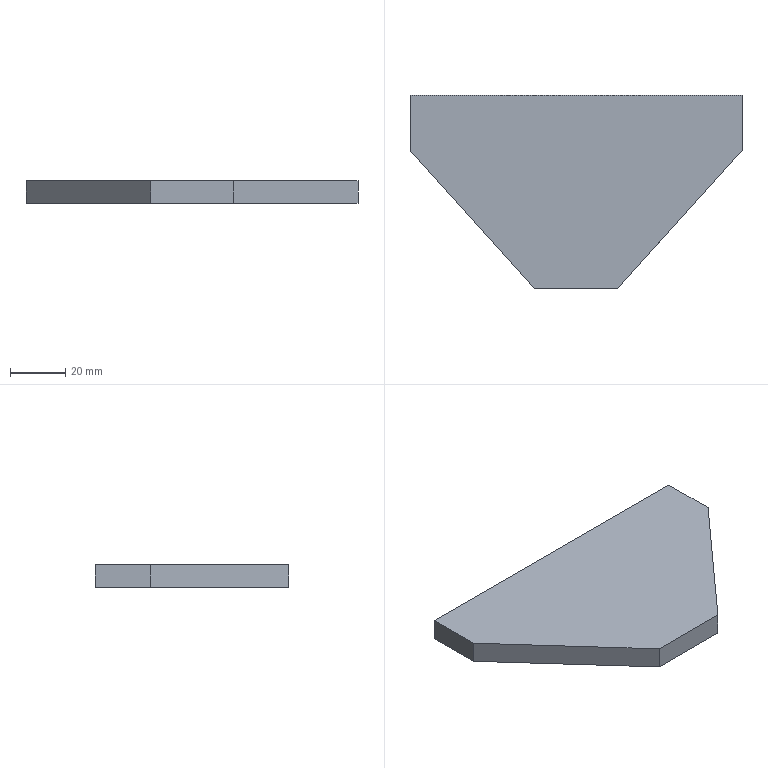Part | SolidWorks | features Extrusion 1, ICE 1 | 1 solid | 8 faces | box 120 x 70 x 8 mm | volume 49200 mm3 | plane 8
STEP:
#1=CARTESIAN_POINT('',(60.,15.,8.));
#2=VERTEX_POINT('',#1);
#3=CARTESIAN_POINT('',(60.,35.,8.));
#4=VERTEX_POINT('',#3);
#5=CARTESIAN_POINT('',(60.,35.,8.));
#6=DIRECTION('',(0.,1.,0.));
#7=VECTOR('',#6,1000.);
#8=LINE('',#5,#7);
#9=EDGE_CURVE('',#2,#4,#8,.T.);
#10=ORIENTED_EDGE('',*,*,#9,.F.);
#11=CARTESIAN_POINT('',(60.,15.,0.));
#12=VERTEX_POINT('',#11);
#13=CARTESIAN_POINT('',(60.,15.,0.));
#14=DIRECTION('',(0.,0.,1.));
#15=VECTOR('',#14,1000.);
#16=LINE('',#13,#15);
#17=EDGE_CURVE('',#12,#2,#16,.T.);
#18=ORIENTED_EDGE('',*,*,#17,.F.);
#19=CARTESIAN_POINT('',(60.,35.,0.));
#20=VERTEX_POINT('',#19);
#21=CARTESIAN_POINT('',(60.,35.,0.));
#22=DIRECTION('',(0.,1.,0.));
#23=VECTOR('',#22,1000.);
#24=LINE('',#21,#23);
#25=EDGE_CURVE('',#12,#20,#24,.T.);
#26=ORIENTED_EDGE('',*,*,#25,.T.);
#27=CARTESIAN_POINT('',(60.,35.,8.));
#28=DIRECTION('',(0.,0.,-1.));
#29=VECTOR('',#28,1000.);
#30=LINE('',#27,#29);
#31=EDGE_CURVE('',#4,#20,#30,.T.);
#32=ORIENTED_EDGE('',*,*,#31,.F.);
#33=EDGE_LOOP('',(#10,#18,#26,#32));
#34=FACE_OUTER_BOUND('',#33,.T.);
#35=CARTESIAN_POINT('',(60.,35.,8.));
#36=DIRECTION('',(-1.,0.,0.));
#37=DIRECTION('',(0.,-1.,0.));
#38=AXIS2_PLACEMENT_3D('',#35,#36,#37);
#39=PLANE('',#38);
#40=ADVANCED_FACE('',(#34),#39,.F.);
#41=CARTESIAN_POINT('',(-60.,35.,0.));
#42=VERTEX_POINT('',#41);
#43=CARTESIAN_POINT('',(-60.,35.,0.));
#44=DIRECTION('',(-1.,0.,0.));
#45=VECTOR('',#44,1000.);
#46=LINE('',#43,#45);
#47=EDGE_CURVE('',#20,#42,#46,.T.);
#48=ORIENTED_EDGE('',*,*,#47,.T.);
#49=CARTESIAN_POINT('',(-60.,35.,8.));
#50=VERTEX_POINT('',#49);
#51=CARTESIAN_POINT('',(-60.,35.,8.));
#52=DIRECTION('',(0.,0.,-1.));
#53=VECTOR('',#52,1000.);
#54=LINE('',#51,#53);
#55=EDGE_CURVE('',#50,#42,#54,.T.);
#56=ORIENTED_EDGE('',*,*,#55,.F.);
#57=CARTESIAN_POINT('',(-60.,35.,8.));
#58=DIRECTION('',(-1.,0.,0.));
#59=VECTOR('',#58,1000.);
#60=LINE('',#57,#59);
#61=EDGE_CURVE('',#4,#50,#60,.T.);
#62=ORIENTED_EDGE('',*,*,#61,.F.);
#63=ORIENTED_EDGE('',*,*,#31,.T.);
#64=EDGE_LOOP('',(#48,#56,#62,#63));
#65=FACE_OUTER_BOUND('',#64,.T.);
#66=CARTESIAN_POINT('',(-60.,35.,8.));
#67=DIRECTION('',(0.,-1.,0.));
#68=DIRECTION('',(0.,0.,-1.));
#69=AXIS2_PLACEMENT_3D('',#66,#67,#68);
#70=PLANE('',#69);
#71=ADVANCED_FACE('',(#65),#70,.F.);
#72=CARTESIAN_POINT('',(-60.,15.,0.));
#73=VERTEX_POINT('',#72);
#74=CARTESIAN_POINT('',(-60.,35.,0.));
#75=DIRECTION('',(0.,-1.,0.));
#76=VECTOR('',#75,1000.);
#77=LINE('',#74,#76);
#78=EDGE_CURVE('',#42,#73,#77,.T.);
#79=ORIENTED_EDGE('',*,*,#78,.T.);
#80=CARTESIAN_POINT('',(-60.,15.,8.));
#81=VERTEX_POINT('',#80);
#82=CARTESIAN_POINT('',(-60.,15.,0.));
#83=DIRECTION('',(0.,0.,1.));
#84=VECTOR('',#83,1000.);
#85=LINE('',#82,#84);
#86=EDGE_CURVE('',#73,#81,#85,.T.);
#87=ORIENTED_EDGE('',*,*,#86,.T.);
#88=CARTESIAN_POINT('',(-60.,35.,8.));
#89=DIRECTION('',(0.,-1.,0.));
#90=VECTOR('',#89,1000.);
#91=LINE('',#88,#90);
#92=EDGE_CURVE('',#50,#81,#91,.T.);
#93=ORIENTED_EDGE('',*,*,#92,.F.);
#94=ORIENTED_EDGE('',*,*,#55,.T.);
#95=EDGE_LOOP('',(#79,#87,#93,#94));
#96=FACE_OUTER_BOUND('',#95,.T.);
#97=CARTESIAN_POINT('',(-60.,35.,8.));
#98=DIRECTION('',(1.,0.,0.));
#99=DIRECTION('',(0.,1.,0.));
#100=AXIS2_PLACEMENT_3D('',#97,#98,#99);
#101=PLANE('',#100);
#102=ADVANCED_FACE('',(#96),#101,.F.);
#103=CARTESIAN_POINT('',(-15.,-35.,8.));
#104=VERTEX_POINT('',#103);
#105=CARTESIAN_POINT('',(15.,-35.,8.));
#106=VERTEX_POINT('',#105);
#107=CARTESIAN_POINT('',(-60.,-35.,8.));
#108=DIRECTION('',(1.,0.,0.));
#109=VECTOR('',#108,1000.);
#110=LINE('',#107,#109);
#111=EDGE_CURVE('',#104,#106,#110,.T.);
#112=ORIENTED_EDGE('',*,*,#111,.F.);
#113=CARTESIAN_POINT('',(-15.,-35.,0.));
#114=VERTEX_POINT('',#113);
#115=CARTESIAN_POINT('',(-15.,-35.,0.));
#116=DIRECTION('',(0.,0.,1.));
#117=VECTOR('',#116,1000.);
#118=LINE('',#115,#117);
#119=EDGE_CURVE('',#114,#104,#118,.T.);
#120=ORIENTED_EDGE('',*,*,#119,.F.);
#121=CARTESIAN_POINT('',(15.,-35.,0.));
#122=VERTEX_POINT('',#121);
#123=CARTESIAN_POINT('',(-60.,-35.,0.));
#124=DIRECTION('',(1.,0.,0.));
#125=VECTOR('',#124,1000.);
#126=LINE('',#123,#125);
#127=EDGE_CURVE('',#114,#122,#126,.T.);
#128=ORIENTED_EDGE('',*,*,#127,.T.);
#129=CARTESIAN_POINT('',(15.,-35.,0.));
#130=DIRECTION('',(0.,0.,1.));
#131=VECTOR('',#130,1000.);
#132=LINE('',#129,#131);
#133=EDGE_CURVE('',#122,#106,#132,.T.);
#134=ORIENTED_EDGE('',*,*,#133,.T.);
#135=EDGE_LOOP('',(#112,#120,#128,#134));
#136=FACE_OUTER_BOUND('',#135,.T.);
#137=CARTESIAN_POINT('',(-60.,-35.,8.));
#138=DIRECTION('',(0.,1.,0.));
#139=DIRECTION('',(0.,0.,1.));
#140=AXIS2_PLACEMENT_3D('',#137,#138,#139);
#141=PLANE('',#140);
#142=ADVANCED_FACE('',(#136),#141,.F.);
#143=CARTESIAN_POINT('',(-60.,15.,8.));
#144=DIRECTION('',(-0.669,0.7433,0.));
#145=VECTOR('',#144,1000.);
#146=LINE('',#143,#145);
#147=EDGE_CURVE('',#104,#81,#146,.T.);
#148=ORIENTED_EDGE('',*,*,#147,.F.);
#149=ORIENTED_EDGE('',*,*,#111,.T.);
#150=CARTESIAN_POINT('',(15.,-35.,8.));
#151=DIRECTION('',(-0.669,-0.7433,0.));
#152=VECTOR('',#151,1000.);
#153=LINE('',#150,#152);
#154=EDGE_CURVE('',#2,#106,#153,.T.);
#155=ORIENTED_EDGE('',*,*,#154,.F.);
#156=ORIENTED_EDGE('',*,*,#9,.T.);
#157=ORIENTED_EDGE('',*,*,#61,.T.);
#158=ORIENTED_EDGE('',*,*,#92,.T.);
#159=EDGE_LOOP('',(#148,#149,#155,#156,#157,#158));
#160=FACE_OUTER_BOUND('',#159,.T.);
#161=CARTESIAN_POINT('',(0.,0.,8.));
#162=DIRECTION('',(0.,0.,1.));
#163=DIRECTION('',(1.,0.,0.));
#164=AXIS2_PLACEMENT_3D('',#161,#162,#163);
#165=PLANE('',#164);
#166=ADVANCED_FACE('',(#160),#165,.T.);
#167=ORIENTED_EDGE('',*,*,#127,.F.);
#168=CARTESIAN_POINT('',(-60.,15.,0.));
#169=DIRECTION('',(-0.669,0.7433,0.));
#170=VECTOR('',#169,1000.);
#171=LINE('',#168,#170);
#172=EDGE_CURVE('',#114,#73,#171,.T.);
#173=ORIENTED_EDGE('',*,*,#172,.T.);
#174=ORIENTED_EDGE('',*,*,#78,.F.);
#175=ORIENTED_EDGE('',*,*,#47,.F.);
#176=ORIENTED_EDGE('',*,*,#25,.F.);
#177=CARTESIAN_POINT('',(15.,-35.,0.));
#178=DIRECTION('',(-0.669,-0.7433,0.));
#179=VECTOR('',#178,1000.);
#180=LINE('',#177,#179);
#181=EDGE_CURVE('',#12,#122,#180,.T.);
#182=ORIENTED_EDGE('',*,*,#181,.T.);
#183=EDGE_LOOP('',(#167,#173,#174,#175,#176,#182));
#184=FACE_OUTER_BOUND('',#183,.T.);
#185=CARTESIAN_POINT('',(0.,0.,0.));
#186=DIRECTION('',(0.,0.,1.));
#187=DIRECTION('',(1.,0.,0.));
#188=AXIS2_PLACEMENT_3D('',#185,#186,#187);
#189=PLANE('',#188);
#190=ADVANCED_FACE('',(#184),#189,.F.);
#191=ORIENTED_EDGE('',*,*,#154,.T.);
#192=ORIENTED_EDGE('',*,*,#133,.F.);
#193=ORIENTED_EDGE('',*,*,#181,.F.);
#194=ORIENTED_EDGE('',*,*,#17,.T.);
#195=EDGE_LOOP('',(#191,#192,#193,#194));
#196=FACE_OUTER_BOUND('',#195,.T.);
#197=CARTESIAN_POINT('',(15.,-35.,0.));
#198=DIRECTION('',(-0.7433,0.669,0.));
#199=DIRECTION('',(-0.669,-0.7433,0.));
#200=AXIS2_PLACEMENT_3D('',#197,#198,#199);
#201=PLANE('',#200);
#202=ADVANCED_FACE('',(#196),#201,.F.);
#203=ORIENTED_EDGE('',*,*,#147,.T.);
#204=ORIENTED_EDGE('',*,*,#86,.F.);
#205=ORIENTED_EDGE('',*,*,#172,.F.);
#206=ORIENTED_EDGE('',*,*,#119,.T.);
#207=EDGE_LOOP('',(#203,#204,#205,#206));
#208=FACE_OUTER_BOUND('',#207,.T.);
#209=CARTESIAN_POINT('',(-60.,15.,0.));
#210=DIRECTION('',(0.7433,0.669,0.));
#211=DIRECTION('',(-0.669,0.7433,0.));
#212=AXIS2_PLACEMENT_3D('',#209,#210,#211);
#213=PLANE('',#212);
#214=ADVANCED_FACE('',(#208),#213,.F.);
#215=CLOSED_SHELL('',(#40,#71,#102,#142,#166,#190,#202,#214));
#216=MANIFOLD_SOLID_BREP('',#215);
#217=CARTESIAN_POINT('',(0.,0.,0.));
#218=DIRECTION('',(0.,0.,1.));
#219=DIRECTION('',(1.,0.,0.));
#220=AXIS2_PLACEMENT_3D('',#217,#218,#219);
#221=(LENGTH_UNIT()NAMED_UNIT(*)SI_UNIT(.MILLI.,.METRE.));
#222=UNCERTAINTY_MEASURE_WITH_UNIT(LENGTH_MEASURE(0.00001),#221,'','');
#223=(NAMED_UNIT(*)PLANE_ANGLE_UNIT()SI_UNIT($,.RADIAN.));
#224=(NAMED_UNIT(*)SI_UNIT($,.STERADIAN.)SOLID_ANGLE_UNIT());
#225=(GEOMETRIC_REPRESENTATION_CONTEXT(3)GLOBAL_UNCERTAINTY_ASSIGNED_CONTEXT((#222))GLOBAL_UNIT_ASSIGNED_CONTEXT((#221,#223,#224))REPRESENTATION_CONTEXT('',''));
#226=ADVANCED_BREP_SHAPE_REPRESENTATION('',(#216,#220),#225);